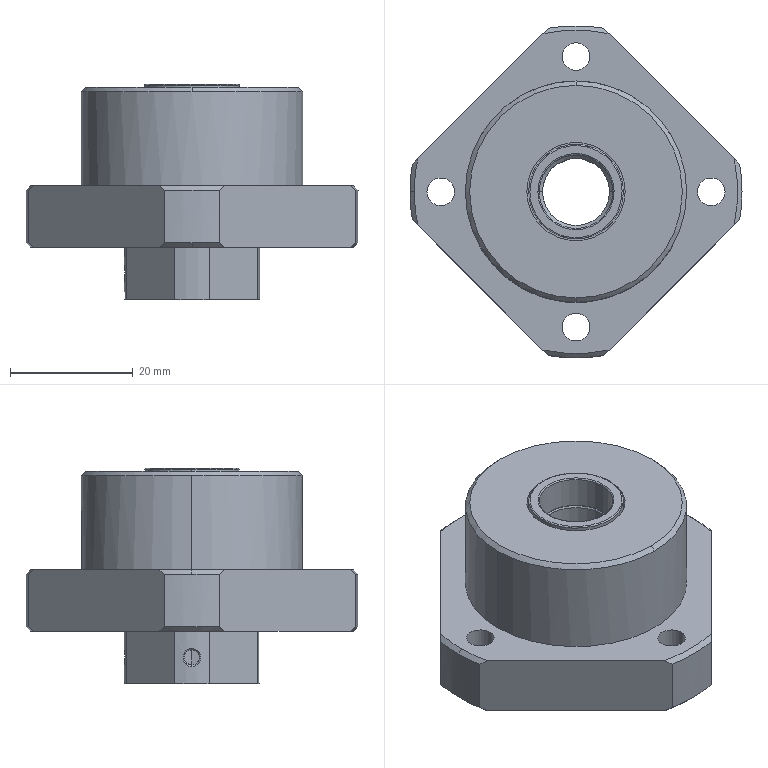Part | SolidWorks | features BaseBody 1 | 1 solid | 120 faces | box 54 x 54 x 35 mm | volume 31856 mm3 | cylinder 52 | cone 25 | plane 23 | spline 20 | commonest cylinder face diameters 4.5 x8 8 x8 12 x6 22 x5 54 x5 2.459 x4